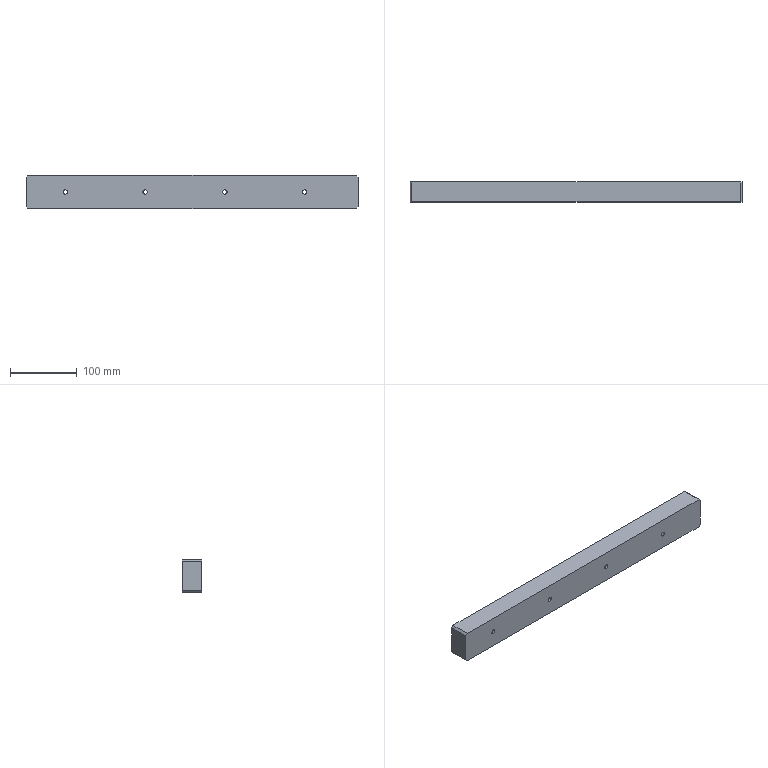Part | SolidWorks | features HoleWzd 2, Chamfer 1, Extrusion 1 | 1 solid | 62 faces | box 499 x 30 x 50 mm | volume 739765 mm3 | cylinder 32 | cone 16 | plane 14 | commonest cylinder face diameters 5 x16 6.6 x8 11 x8